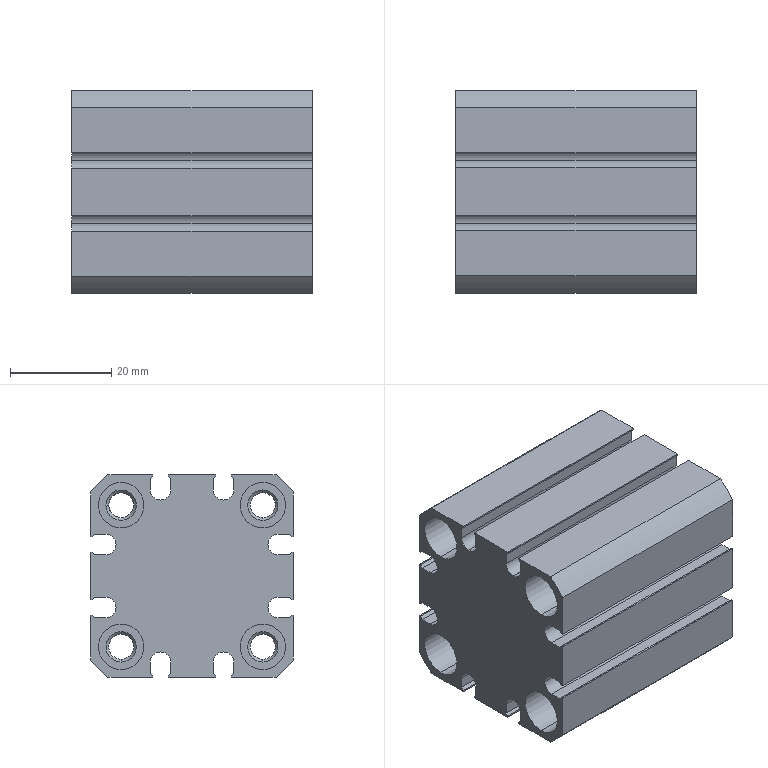Part | STEP file | _MSCCN25-15_c_1 | 1 solid | 213 faces | box 47.5 x 40 x 40 mm | volume 56452 mm3 | plane 89 | cylinder 84 | cone 40 | commonest cylinder face diameters 4 x16 4.917 x16 9 x16 5.5 x8 1.778 x4 4.134 x4